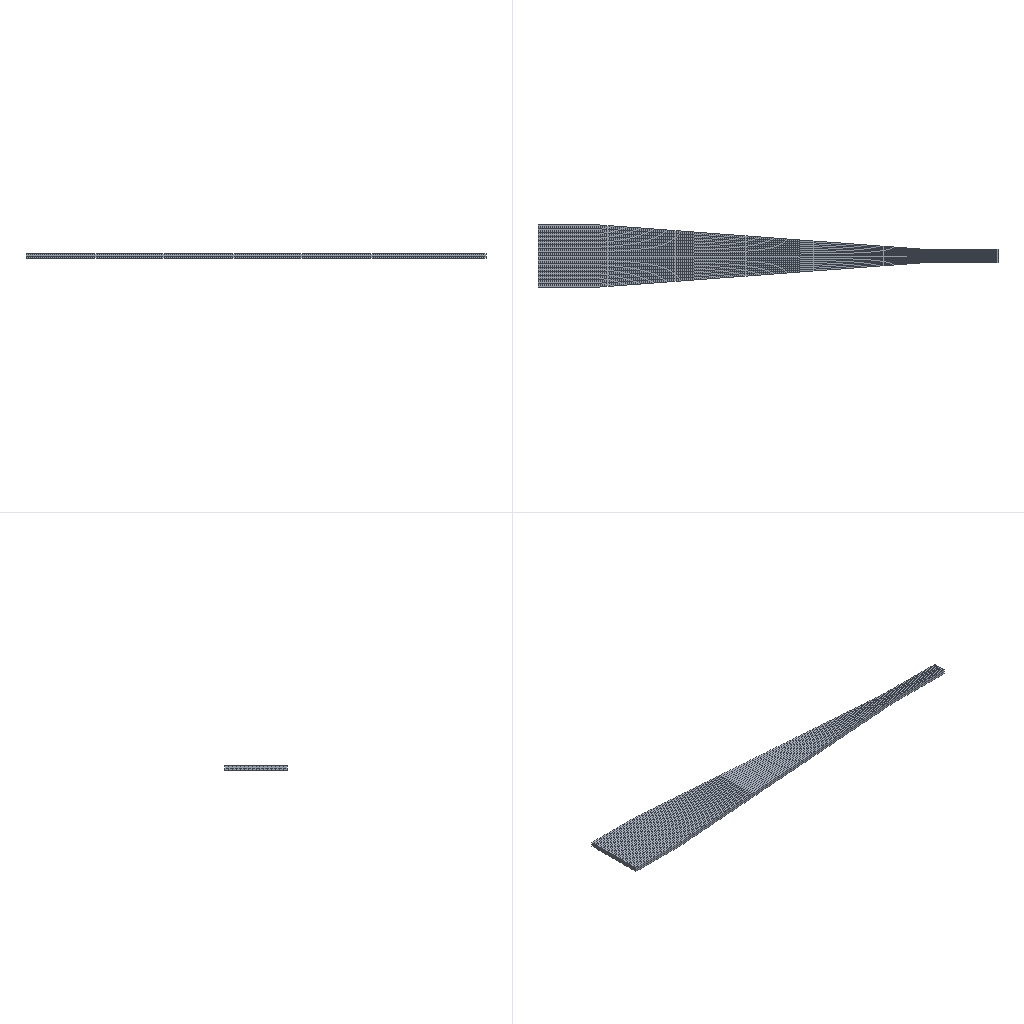Simulation study | abaqus
Set-up summary:
category,name,step,type,value,unit,region
solver,abaqus,,Abaqus/CAE 2024
units,mm-N-s-tonne (MPa),,inferred,E=200000 density=
analysis,Static,,static,time_period=1
mesh,nodes,,,11629
mesh,elements,,,7264
element_type,C3D8R,,,7264
material,Steel,,E,200000
material,Steel,,nu,0.3
section,Steel,,solid section,,,_PickedSet2
load,Load-1,Static,concentrated force,"10 [dir=(0, 0, -1) n=3]",,_PickedSet8
bc,BC-1,Static,encastre,[dofs=ENCASTRE],,_PickedSet4
constraint,coupling,,,1
Abaqus input file, long lists of numbers shortened:
*Heading
** Job name: deck Model name: Model-1
** Generated by: Abaqus/CAE 2024
*Preprint, echo=NO, model=NO, history=NO, contact=NO
**
** PARTS
**
*Part, name=Part-1
*End Part
**
**
** ASSEMBLY
**
*Assembly, name=Assembly
**
*Instance, name=Part-1-1, part=Part-1
*Node
      1,         125.,          -5.,          3.5
      2,        -115.,         -23.,          3.5
** (11626 more lines like these left out)
*Element, type=C3D8R
   1,   688,  1389,  8269,  1359,     1,    19,  1041,   338
   2,  1389,  1390,  8270,  8269,    19,    20,  1042,  1041
** (7262 more lines like these left out)
*Nset, nset=_PickedSet2, internal, generate
     1,  11628,      1
*Elset, elset=_PickedSet2, internal, generate
    1,  7264,     1
** Section: Solid
*Solid Section, elset=_PickedSet2, material=Steel
,
*End Instance
**
*Node
      1,         180.,           0.,           0.
*Nset, nset=_PickedSet4, internal, instance=Part-1-1
     2,     3,     5,     6,     9,    10,    11,    12,    13,    14,   178,   498,   689,   690,   691,   692
   693,   694,   695,   696,   697,   698,   699,   700,   701,   702,   703,   704,   705,   706,   707,   708
** (97 more lines like these left out)
*Elset, elset=_PickedSet4, internal, instance=Part-1-1, generate
 5121,  6080,     1
*Nset, nset=_PickedSet7, internal
 1,
*Nset, nset=_PickedSet8, internal
 1,
*Elset, elset=__PickedSurf6_S2, internal, instance=Part-1-1, generate
 6081,  6112,     1
*Surface, type=ELEMENT, name=_PickedSurf6, internal
__PickedSurf6_S2, S2
** Constraint: Constraint-1
*Coupling, constraint name=Constraint-1, ref node=_PickedSet7, surface=_PickedSurf6
*Kinematic
*End Assembly
**
** MATERIALS
**
*Material, name=Steel
*Elastic
200000., 0.3
** ----------------------------------------------------------------
**
** STEP: Static
**
*Step, name=Static, nlgeom=NO
*Static
1., 1., 1e-05, 1.
**
** BOUNDARY CONDITIONS
**
** Name: BC-1 Type: Symmetry/Antisymmetry/Encastre
*Boundary
_PickedSet4, ENCASTRE
**
** LOADS
**
** Name: Load-1   Type: Concentrated force
*Cload
_PickedSet8, 1, 0.
_PickedSet8, 2, 0.
_PickedSet8, 3, -10.
**
** OUTPUT REQUESTS
**
*Restart, write, frequency=0
**
** FIELD OUTPUT: F-Output-1
**
*Output, field
*Node Output
CF, RF, U
*Element Output, directions=YES
LE, PE, PEEQ, PEMAG, S
**
** HISTORY OUTPUT: H-Output-1
**
*Output, history, variable=PRESELECT
*End Step
Results summary:
result,odb.job_status,,,JOB_STATUS_COMPLETED_SUCCESSFULLY,"consistent, unstated (Abaqus has no unit system)"
result,steps[0].procedure,Static,,*STATIC,"consistent, unstated (Abaqus has no unit system)"
result,steps[0].time_period,Static,,1,"consistent, unstated (Abaqus has no unit system)"
result,steps[0].n_frames,Static,,2,"consistent, unstated (Abaqus has no unit system)"
result,steps[0].last_frame.id,Static,,1,"consistent, unstated (Abaqus has no unit system)"
result,steps[0].last_frame.value,Static,,1,"consistent, unstated (Abaqus has no unit system)"
result,steps[0].last_frame.description,Static,,Increment      1: Step Time =    1.000,"consistent, unstated (Abaqus has no unit system)"
result,steps[0].completed,Static,,True,"consistent, unstated (Abaqus has no unit system)"
result,steps[0].max_U_magnitude,Static,,4.951,"consistent, unstated (Abaqus has no unit system)"
result,steps[0].max_S_mises,Static,,21.956,"consistent, unstated (Abaqus has no unit system)"
result,steps[0].RF_sum[1],Static,,-3.24253e-05,"consistent, unstated (Abaqus has no unit system)"
result,steps[0].RF_sum[2],Static,,9.4946e-07,"consistent, unstated (Abaqus has no unit system)"
result,steps[0].RF_sum[3],Static,,10,"consistent, unstated (Abaqus has no unit system)"